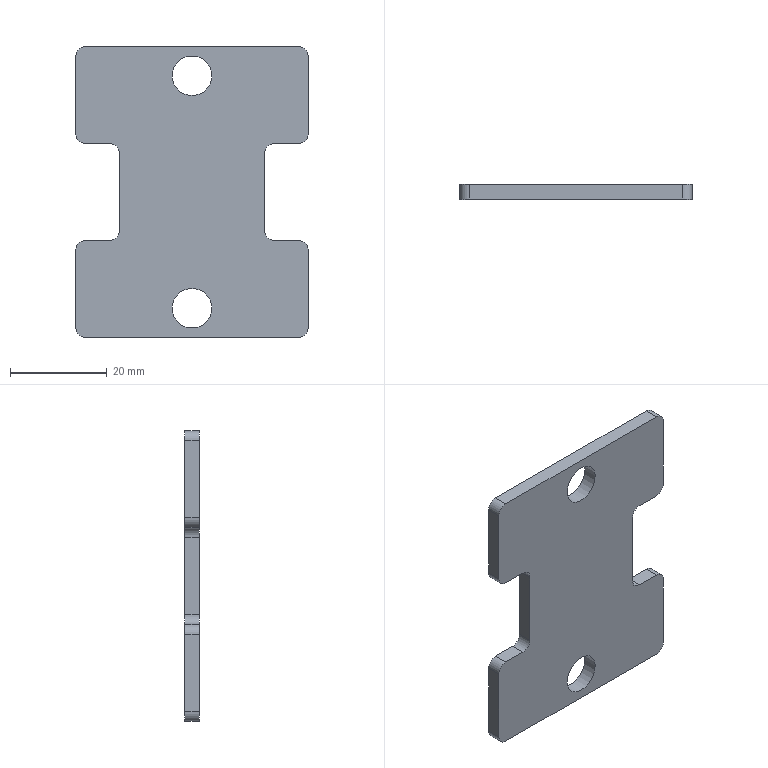Part | STEP file | Connector crossbar | 1 solid | 28 faces | box 48 x 3 x 60 mm | volume 7233 mm3 | cylinder 14 | plane 14 | commonest cylinder face diameters 4 x12 8.2 x2